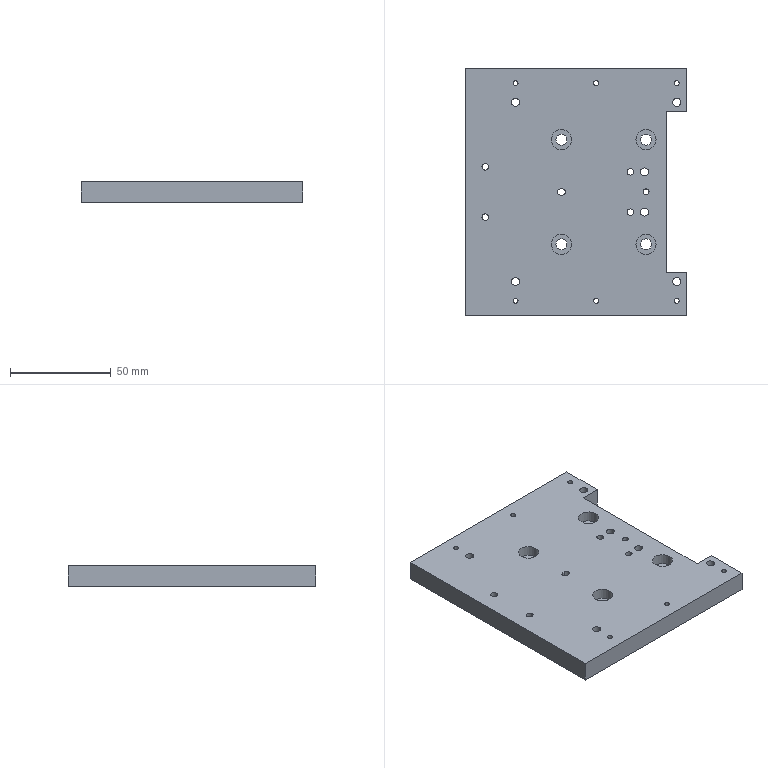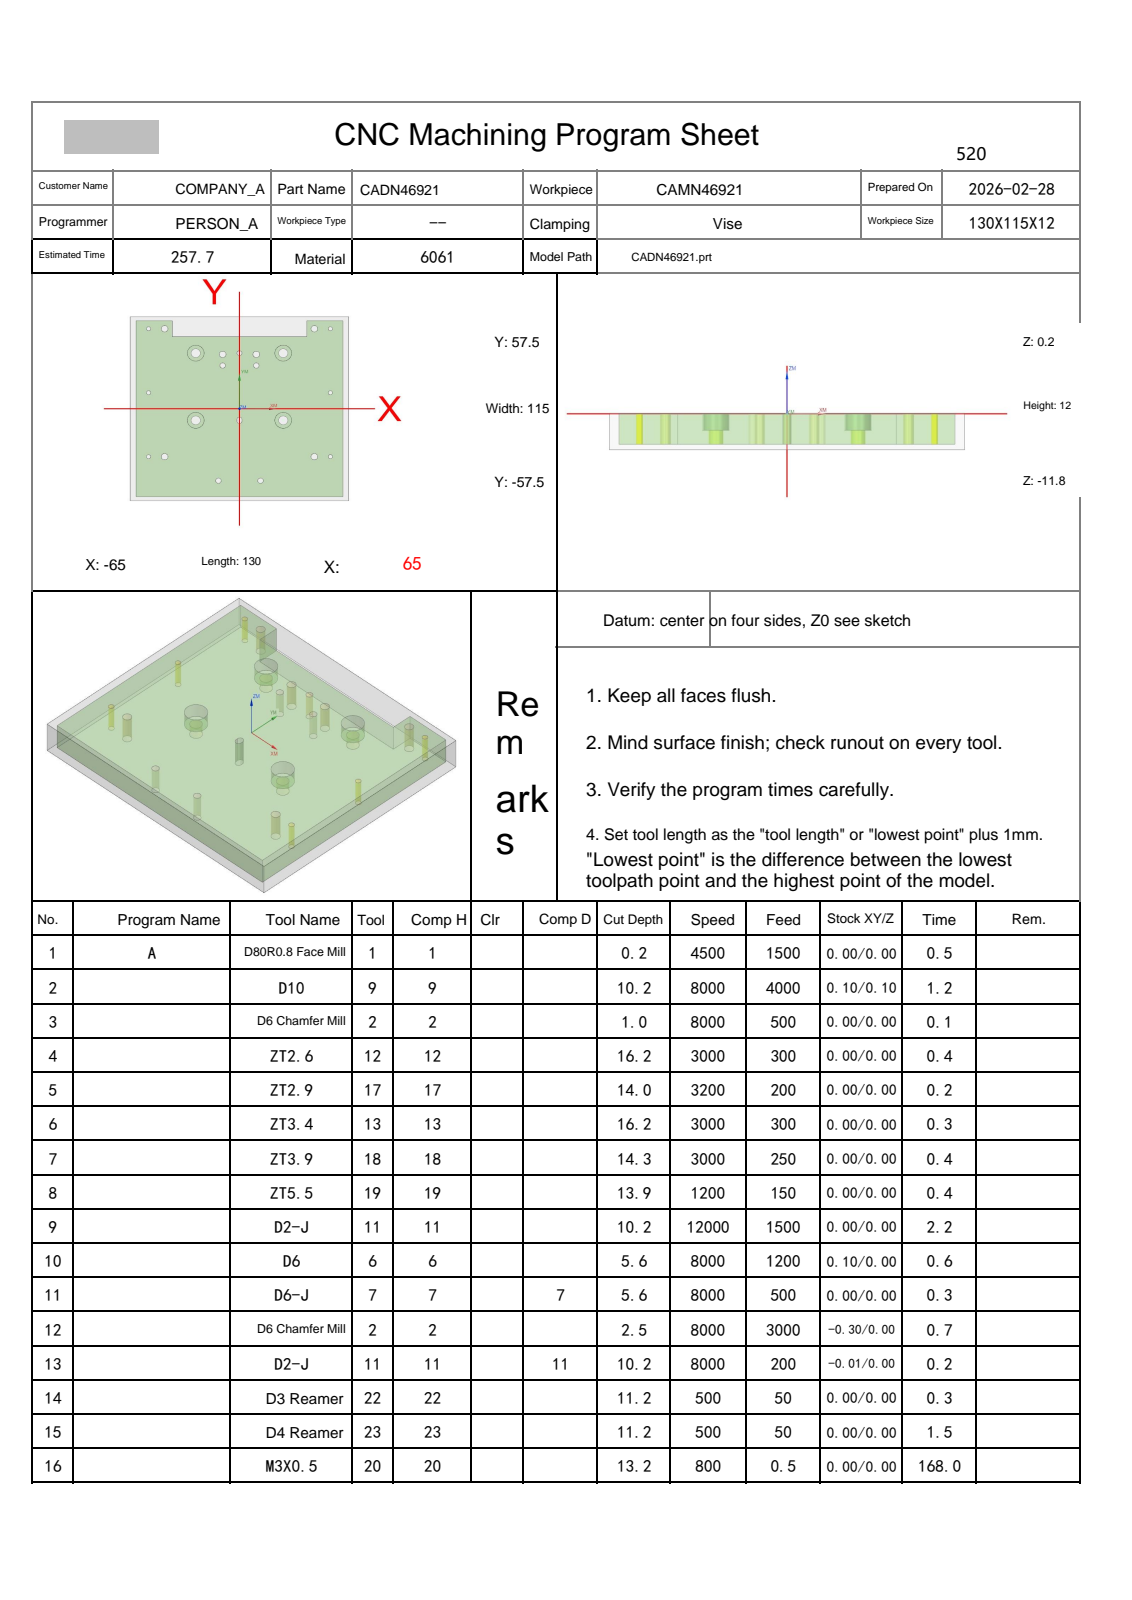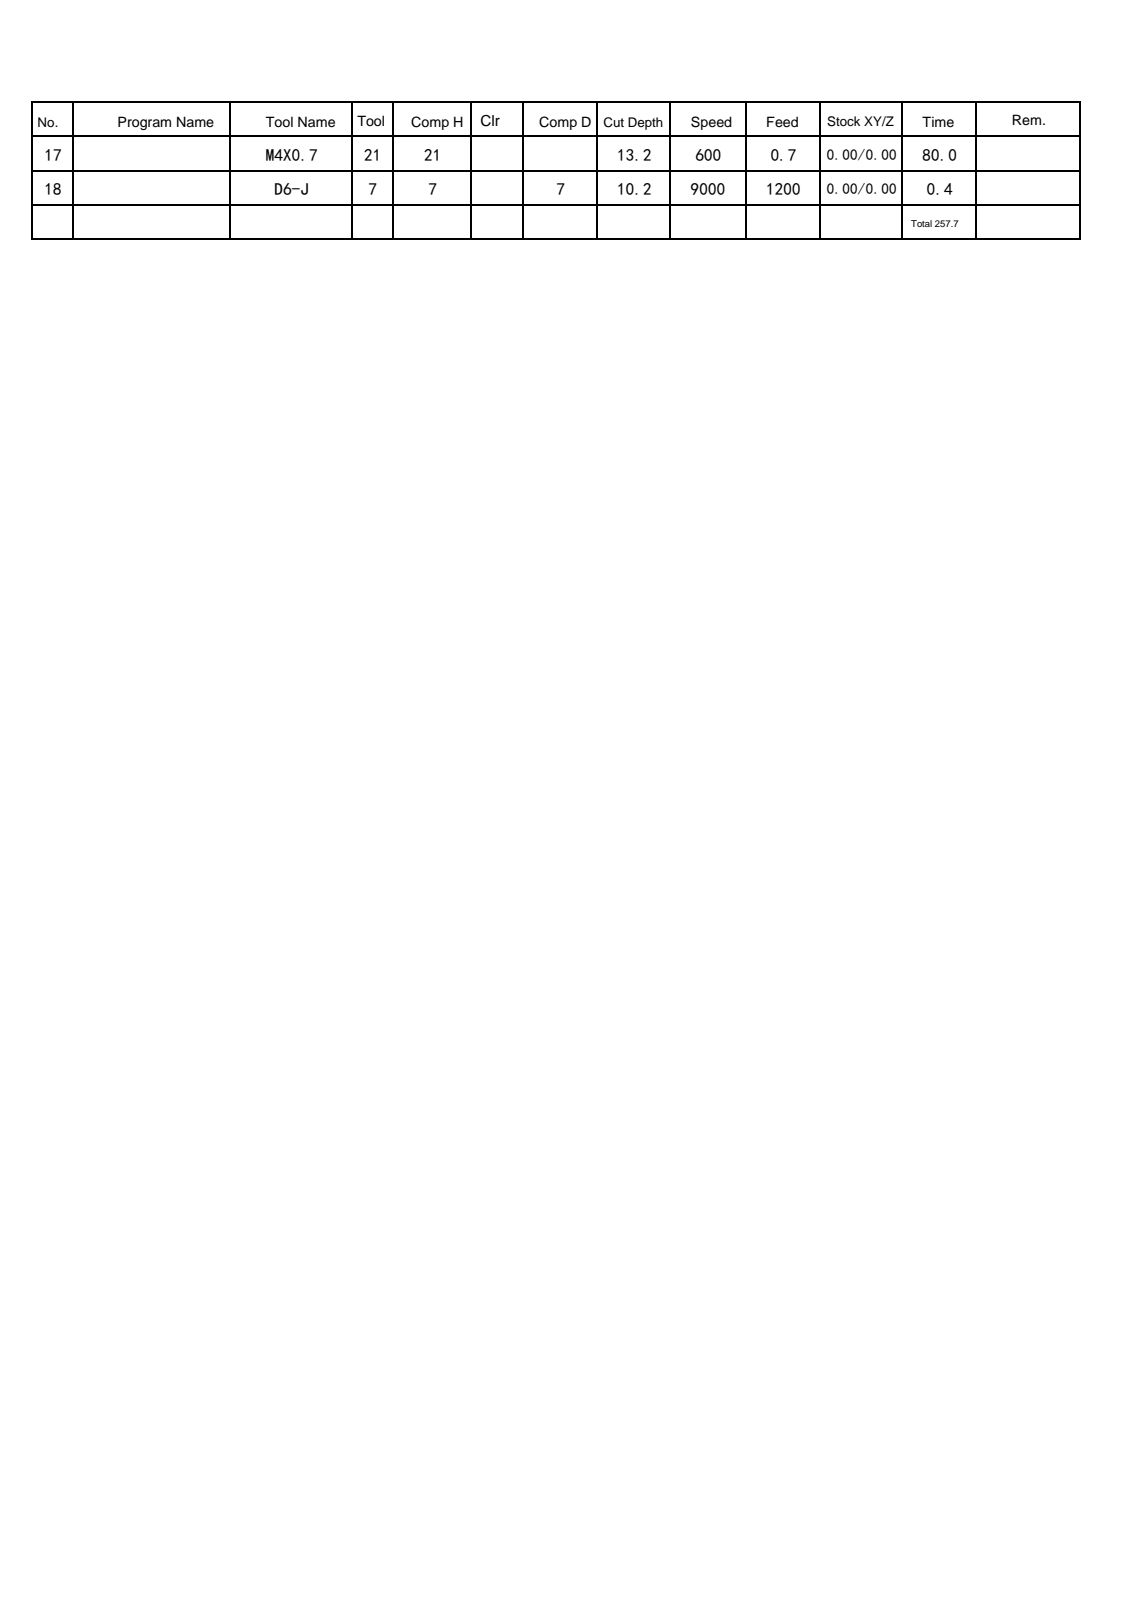NC program | NX | posted by the shop | part box 110 x 123 x 10 mm
Lines 1 to 794 of 4511:
%
O0001
(Machine time: 491.53 MIN)
(===Total Tool:15===)
(T1=D80R0.8 Face Mill D=80.  R=0.8  D-  H01 Z=-0.   )
(T9=D10     D=10.  R=0.   D-  H09 Z=-10.  )
(T2=D6 Chamfer Mill   D=6.   R=0.   D-  H02 Z=-2.3  )
(T12=ZT2.6  D=2.6  DR_a=118 D-  H12 Z=-16.  )
(T17=ZT2.9  D=2.9  DR_a=120 D-  H17 Z=-13.84)
(T13=ZT3.4  D=3.4  DR_a=118 D-  H13 Z=-16.  )
(T18=ZT3.9  D=3.9  DR_a=120 D-  H18 Z=-14.13)
(T19=ZT5.5  D=5.5  DR_a=118 D-  H19 Z=-13.65)
(T11=D2-J   D=2.   R=0.   D-  H11 Z=-10.  )
(T6=D6      D=6.   R=0.   D-  H06 Z=-5.4  )
(T7=D6-J    D=6.   R=0.   D7  H07 Z=-10.  )
(T22=D3 Reamer   D=3.   DR_a=180 D22 H22 Z=-11.  )
(T23=D4 Reamer   D=4.   DR_a=180 D-  H23 Z=-11.  )
(T20=M3X0.5 D=2.5  DR_a=180 D-  H20 Z=-13.  )
(T21=M4X0.7 D=3.3  DR_a=180 D-  H21 Z=-13.  )
G80 G90 G17 G49 G40
G91 G28 Z0
M01
N1 T01 M06
(D80R0.8 Face Mill  D=80. R=0.8 H=01 ce=0.00 di=0.00)
G00 G90 G54 X106.5 Y-47.5 M03 S4500
G43 H01 Z50.
M08
Z2.
G01 Z0.0 F1500.
X101.5
X-101.5
Y0.0
X101.5
Y47.5
X-101.5
X-106.5
Z2.
G00 Z50.
G91 G28 Z0.0
M05
M09
G91 G28 Z0.0
M01
N2 T09 M06
(D10  D=10. R=0. H=09 ce=0.10 di=0.10)
G00 G90 G54 X62.505 Y-68.93 M03 S8000
G43 H09 Z50.
M08
Z-8.
G01 X62.486 Y-68.832 Z-8.625 F4000.
X62.467 Y-68.734 Z-8.872
X62.448 Y-68.636 Z-9.054
X62.43 Y-68.538 Z-9.2
X62.411 Y-68.439 Z-9.323
X62.392 Y-68.341 Z-9.428
X62.374 Y-68.243 Z-9.52
X62.355 Y-68.145 Z-9.6
X62.336 Y-68.046 Z-9.67
X62.318 Y-67.948 Z-9.732
X62.299 Y-67.85 Z-9.786
X62.28 Y-67.752 Z-9.833
X62.261 Y-67.653 Z-9.874
X62.243 Y-67.555 Z-9.908
X62.224 Y-67.457 Z-9.936
X62.205 Y-67.359 Z-9.96
X62.187 Y-67.26 Z-9.977
X62.168 Y-67.162 Z-9.99
X62.149 Y-67.064 Z-9.997
X62.131 Y-66.966 Z-10.
X61.728 Y-64.851
G03 X61.47 Y-64.5 I-.505 J-.101
X57.665 Y-63.862 I-4.014 J-12.282
X48.447 Y-63.687 I-9.217 J-242.545
X45.931 Y-63.7 I0.0 J-242.72
G01 X-63.188 Y-63.681
G02 X-69.789 Y-59.121 I.026 J7.095
X-71.019 Y-52.954 I17.461 J6.69
X-71.212 Y-43.817 I217.094 J9.136
X-71.199 Y-41.437 I217.286 J0.0
G01 X-71.177 Y55.743
G02 X-66.615 Y62.297 I7.094 J-.073
X-60.526 Y63.515 I6.642 J-17.363
X-51.392 Y63.712 I9.134 J-212.235
X-49.009 Y63.699 I0.0 J-212.431
G01 X63.29 Y63.675
G02 X69.773 Y59.159 I-.116 J-7.078
X70.995 Y53.307 I-16.699 J-6.54
X71.216 Y43.947 I-197.872 J-9.36
X71.199 Y41.31 I-198.093 J0.0
G01 X71.175 Y-55.789
G02 X66.602 Y-62.298 I-7.094 J.123
X62.072 Y-63.143 I-4.53 J11.728
X61.502 Y-63.13 I0.0 J12.572
G03 X44.885 Y-62.897 I-16.617 J-593.259
X42.812 Y-62.901 I0.0 J-593.491
G01 X-61.328 Y-62.88
G02 X-68.312 Y-58.453 I.17 J7.991
X-70.034 Y-52.247 I15.045 J7.518
X-70.398 Y-43.651 I101.199 J8.596
X-70.39 Y-42.338 I101.564 J0.0
G01 X-70.376 Y53.887
G02 X-65.947 Y60.818 I7.979 J-.217
X-59.657 Y62.545 I7.553 J-15.196
X-51.066 Y62.899 I8.592 J-104.056
X-49.748 Y62.89 I0.0 J-104.41
G01 X61.347 Y62.878
G02 X68.339 Y58.403 I-.195 J-8.003
X70.05 Y52.108 I-15.333 J-7.548
X70.399 Y43.512 I-105.559 J-8.596
X70.391 Y42.198 I-105.908 J0.0
G01 X70.378 Y-53.847
G02 X65.26 Y-61.016 I-7.763 J.131
X59.223 Y-62.088 I-6.136 J17.023
X52.104 Y-62.14 I-7.119 J496.003
X46.088 Y-62.103 I0.0 J496.054
G01 X-59.568 Y-62.078
G02 X-67.383 Y-57.053 I.237 J8.959
X-69.224 Y-50.22 I16.92 J8.222
X-69.6 Y-40.954 I113.845 J9.266
X-69.591 Y-39.51 I114.221 J0.0
G01 X-69.579 Y51.99
G02 X-64.471 Y59.933 I8.996 J-.171
X-57.46 Y61.754 I8.273 J-17.449
X-47.647 Y62.11 I9.813 J-135.265
X-45.629 Y62.095 I0.0 J-135.62
G01 X59.55 Y62.077
G02 X67.333 Y57.147 I-.205 J-8.932
X69.203 Y50.405 I-16.458 J-8.195
X69.601 Y41.071 I-109.254 J-9.334
X69.59 Y39.537 I-109.652 J0.0
G01 X69.581 Y-51.963
G02 X64.414 Y-59.706 I-8.458 J.049
X58.127 Y-61.133 I-7.21 J17.206
X50.107 Y-61.327 I-8.02 J165.472
X47.368 Y-61.304 I0.0 J165.666
G01 X-57.808 Y-61.277
G02 X-62.753 Y-59.935 I.161 J10.372
G01 X-64.05 Y-59.417
X-65.106 Y-58.606
G02 X-67.093 Y-55.012 I8.097 J6.822
X-68.555 Y-47.093 I26.837 J9.048
X-68.814 Y-36.113 I232.394 J10.979
X-68.797 Y-33.337 I232.653 J0.0
G01 X-68.775 Y50.322
G02 X-66.234 Y56.812 I9.75 J-.075
G01 X-65.834 Y57.688
G02 X-63.98 Y59.456 I4.92 J-3.302
X-60.748 Y60.372 I4.831 J-10.887
X-50.156 Y61.25 I10.591 J-63.457
G01 X-49.837 Y61.249
X-37.837 Y61.298
X57.823 Y61.275
G02 X62.751 Y59.935 I-.18 J-10.397
G01 X64.05 Y59.417
X65.106 Y58.606
G02 X67.148 Y54.861 I-8.31 J-6.961
X68.566 Y46.933 I-27.584 J-9.022
X68.813 Y36.045 I-239.895 J-10.888
X68.797 Y33.337 I-240.142 J0.0
G01 X68.775 Y-50.322
G02 X66.395 Y-56.45 I-9.386 J.12
X65.02 Y-58.691 I-5.677 J1.941
X62.781 Y-59.936 I-3.933 J4.432
X53.648 Y-60.466 I-9.133 J78.497
G01 X53.498
X45.258 Y-60.501
X-55.922 Y-60.484
G02 X-59.036 Y-60.1 I.36 J15.741
G01 X-61.502
X-62.771 Y-59.933
X-61.502 Y-60.1
X61.5
G03 X63.98 Y-59.456 I-.213 J5.922
X65.834 Y-57.688 I-3.066 J5.071
X67.744 Y-51.783 I-20.321 J9.836
X68.146 Y-44.982 I-57.397 J6.801
X68.14 Y-44.199 I-57.799 J0.0
G01 X68.134 Y39.461
G03 X68.139 Y40.356 I-79.496 J.895
X67.562 Y49.917 I-79.501 J0.0
X66.6 Y54.052 I-26.021 J-3.876
X66.607 Y54.435 I-9.886 J.383
X66.426 Y56.32 I-9.894 J0.0
G01 X65.917 Y57.55
X66.426 Y56.32
G02 X66.624 Y53.695 I-17.291 J-2.625
X66.6 Y52.772 I-17.49 J0.0
X67.229 Y43.406 I-241.196 J-20.908
X67.366 Y30.259 I-629.886 J-13.147
X67.358 Y26.927 I-630.024 J0.0
G01 X67.334 Y-43.933
G02 X67.34 Y-44.665 I-46.782 J-.732
X66.871 Y-51.27 I-46.788 J0.0
G01 X66.6 Y-52.569
G02 X66.62 Y-53.631 I-28.416 J-1.062
X66.537 Y-55.798 I-28.436 J0.0
G01 X66.373 Y-56.499
G03 X66.6 Y-55.001 I-5.982 J1.672
G01 Y-54.736
G02 X66.708 Y-40.418 I945.397 J0.0
G01 X66.693 Y37.241
G02 X66.585 Y48.543 I590.334 J11.301
X66.6 Y52.803 I590.442 J0.0
G01 Y-48.957
G03 X67.1 Y-49.457 I.5 J0.0
X67.513 Y-49.239 I0.0 J.5
G01 X67.947 Y-48.602
X69.057 Y-46.972 Z-9.9
X69.65 Y-46.102
X69.687 Y-46.037
X69.715 Y-45.967
X69.731 Y-45.895
X69.737 Y-45.82
Y55.954
X69.73 Y56.211
X69.71 Y56.468
X69.677 Y56.724
X69.631 Y56.977
X69.571 Y57.228
X69.499 Y57.475
X69.414 Y57.718
X69.316 Y57.957
X69.206 Y58.19
X69.085 Y58.417
X68.951 Y58.638
X68.807 Y58.851
X68.652 Y59.057
X67.036 Y61.084
X66.983 Y61.141
X66.921 Y61.189
X66.853 Y61.227
X66.78 Y61.253
X66.703 Y61.268
X66.625 Y61.271
X66.548 Y61.262
X66.473 Y61.241
X65.994 Y61.066
X64.144 Y60.386 Z-10.
X62.911 Y59.94
X59.239 Y60.42
G03 X50.912 Y60.673 I-8.327 J-136.576
X48.684 Y60.655 I0.0 J-136.83
G01 X-45.841 Y60.645
G03 X-47.114 Y60.652 I-1.274 J-108.167
X-57.504 Y60.152 I0.0 J-108.175
G01 X-57.928 Y60.1
X-61.498
X-62.781 Y59.936
X-61.498 Y60.1
X-39.725 Y60.075
G03 X-31.255 Y59.847 I8.47 J156.731
X-29.209 Y59.86 I0.0 J156.96
G01 X38.547 Y59.878
G02 X40.002 Y60.1 I3.204 J-16.087
G01 X61.502
X62.295 Y59.995
X62.36 Y59.991
G03 X62.86 Y60.491 I0.0 J.5
X62.623 Y60.916 I-.5 J0.0
G01 X61.653 Y61.517
X59.977 Y62.556 Z-9.9
X59.8 Y62.665
X59.742 Y62.696
X59.68 Y62.719
X59.616 Y62.734
X59.55 Y62.74
X40.521 Y63.247
X40.436 Y63.242
X40.353 Y63.222
X40.275 Y63.189
X40.203 Y63.143
X40.14 Y63.086
X40.088 Y63.019
X40.048 Y62.944
X39.893 Y62.583
X39.115 Y60.771 Z-10.
X38.812 Y60.081
G02 X37.832 Y59.658 I-1.101 J1.202
X32.456 Y59.247 I-5.376 J34.946
X31.849 Y59.252 I0.0 J35.358
G01 X22.871 Y59.218
X-33.56 Y59.243
X-37.29 Y59.346
X-38.68 Y59.926
X-39.998 Y60.1
X-38.68 Y59.926
G03 X-36.585 Y59.055 I11.251 J24.099
X-31.218 Y58.497 I5.367 J25.538
G01 X-31.088
G03 X-20.883 Y58.417 I10.205 J646.307
X-19.532 Y58.418 I0.0 J646.388
G01 X30.574 Y58.444
G03 X31.065 Y58.441 I.492 J44.925
X36.555 Y58.778 I0.0 J44.928
X37.45 Y59.417 I-3.02 J5.179
G01 X38.485 Y59.845
G03 X36.58 Y58.757 I1.486 J-4.809
G02 X33.107 Y58.014 I-3.831 J9.425
X24.641 Y57.766 I-8.466 J144.323
X22.707 Y57.779 I0.0 J144.571
G01 X-27.719 Y57.804
G02 X-28.459 Y57.798 I-.74 J51.357
X-35.172 Y58.239 I0.0 J51.362
X-36.394 Y58.606 I.167 J2.77
G01 X-37.409 Y59.385
G03 X-35.849 Y58.211 I9.538 J11.048
X-31.824 Y57.286 I4.687 J11.178
X-23.321 Y56.978 I8.503 J117.162
X-22.001 Y56.985 I0.0 J117.47
G01 X26.58 Y57.001
G03 X27.394 Y56.995 I.814 J51.142
X34.203 Y57.45 I0.0 J51.148
X35.877 Y57.95 I-.524 J4.802
G02 X36.648 Y58.801 I3.084 J-2.019
G03 X35.817 Y57.87 I2.562 J-3.122
G02 X32.885 Y56.843 I-3.666 J5.766
X25.432 Y56.36 I-7.453 J57.247
X24.665 Y56.365 I0.0 J57.73
G01 X-22.542 Y56.35
G02 X-23.837 Y56.34 I-1.295 J84.158
X-32.198 Y56.757 I0.0 J84.168
X-35.682 Y57.718 I.883 J9.996
G01 X-36.355 Y58.556
G03 X-35.092 Y57.208 I3.927 J2.413
X-31.072 Y56.023 I5.06 J9.756
X-22.39 Y55.553 I8.681 J79.953
X-21.422 Y55.559 I0.0 J80.422
G01 X23.938 Y55.564
G03 X24.727 Y55.558 I.789 J57.881
X32.378 Y56.066 I0.0 J57.886
X35.293 Y57.018 I-1.102 J8.313
X35.583 Y57.55 I-1.475 J1.151
G01 X35.875 Y57.931
G03 X35.374 Y57.065 I1.947 J-1.707
G02 X32.939 Y55.801 I-3.455 J3.676
X26.378 Y55.018 I-6.847 J29.497
X16.15 Y54.895 I-10.228 J425.475
X14.228 Y54.899 I0.0 J425.598
G01 X-21.483 Y54.924
G02 X-22.293 Y54.919 I-.809 J72.281
X-30.925 Y55.436 I0.0 J72.285
X-34.897 Y56.658 I1.245 J11.119
X-35.583 Y57.55 I.614 J1.182
G01 X-35.681 Y57.677
G02 X-35.32 Y56.926 I-3.681 J-2.23
G03 X-33.019 Y55.424 I3.621 J3.034
X-26.761 Y54.346 I7.101 J22.511
X-16.524 Y54.093 I10.237 J206.976
X-14.649 Y54.101 I0.0 J207.229
G01 X21.698 Y54.126
G03 X22.408 Y54.122 I.711 J65.855
X30.737 Y54.651 I0.0 J65.858
X34.774 Y56.016 I-1.098 J9.897
X35.074 Y56.32 I-2.438 J2.705
G01 X35.441 Y57.207
G02 X34.923 Y56.066 I-4.848 J1.512
X32.248 Y54.565 I-4.032 J4.054
X25.829 Y53.643 I-7.141 J26.887
X15.924 Y53.454 I-9.905 J260.528
X14.148 Y53.46 I0.0 J260.716
G01 X-19.322 Y53.486
G02 X-20.139 Y53.481 I-.816 J78.127
X-29.49 Y54.043 I0.0 J78.132
X-34.258 Y55.54 I1.366 J12.694
X-35.074 Y56.32 I.733 J1.583
G01 X-35.38 Y57.059
G03 X-34.85 Y55.836 I6.316 J2.011
X-31.93 Y54.043 I4.58 J4.184
X-24.941 Y52.904 I7.952 J26.768
X-12.517 Y52.637 I12.424 J289.718
X-8.892 Y52.66 I0.0 J289.984
G01 X19.934 Y52.69
G03 X20.601 Y52.687 I.667 J68.704
X29.603 Y53.279 I0.0 J68.708
X34.042 Y54.754 I-1.455 J11.799
X34.994 Y55.713 I-.967 J1.912
G01 X35.074 Y56.32
Y56.271
G02 X34.182 Y54.6 I-2.011 J0.0
X29.919 Y52.853 I-5.859 J8.225
X21.099 Y52.093 I-8.82 J50.778
G01 X21.09
X12.549 Y52.02
X-17.402 Y52.048
G02 X-18.149 Y52.044 I-.747 J85.721
X-28.074 Y52.621 I0.0 J85.724
X-33.372 Y54.176 I1.684 J15.538
X-34.972 Y55.605 I1.598 J3.398
G01 X-35.074 Y56.32
Y56.314
G03 X-33.953 Y54.175 I2.602 J0.0
X-29.412 Y52.234 I6.527 J8.987
X-20.52 Y51.337 I9.338 J48.079
X-9.772 Y51.22 I11.644 J577.468
G01 X18.173 Y51.252
G03 X18.776 Y51.25 I.602 J75.544
X28.35 Y51.859 I0.0 J75.546
X33.518 Y53.519 I-1.643 J13.992
X34.868 Y54.781 I-1.808 J3.286
G01 X34.984 Y55.636
G02 X34.814 Y54.568 I-3.95 J.082
X32.508 Y52.601 I-4.19 J2.574
X26.353 Y51.058 I-7.671 J17.558
X15.687 Y50.584 I-10.666 J119.748
X14.208 Y50.593 I0.0 J120.222
G01 X-15.18 Y50.607
G02 X-16.067 Y50.602 I-.887 J96.053
X-26.963 Y51.222 I0.0 J96.058
X-32.769 Y52.896 I1.904 J17.516
X-34.874 Y54.772 I2.044 J4.412
G01 X-34.983 Y55.633
G03 X-34.774 Y54.376 I4.726 J.142
X-32.255 Y52.125 I4.726 J2.753
X-25.853 Y50.395 I8.298 J18.003
G01 X-22.925 Y50.1
X23.646 Y50.123
G03 X31.233 Y51.408 I-.56 J26.332
X34.563 Y53.509 I-2.269 J7.284
X34.9 Y54.135 I-1.094 J.994
G01 Y54.855
G02 X34.925 Y54.506 I-2.424 J-.349
X34.745 Y53.583 I-2.449 J0.0
X32.224 Y51.407 I-4.761 J2.965
X28.178 Y50.1 I-6.943 J14.582
G01 X23.058
X29.646 Y50.125
G03 X34.562 Y52.602 I-.644 J7.395
X34.9 Y53.234 I-1.322 J1.114
G01 Y54.114
G02 X34.921 Y53.713 I-3.914 J-.401
X34.829 Y52.867 I-3.935 J0.0
X32.55 Y50.629 I-4.308 J2.106
X31.261 Y50.1 I-4.205 J8.411
G01 X29.261
G03 X30.191 Y50.082 I.93 J23.649
X31.947 Y50.147 I0.0 J23.667
X34.866 Y52.224 I-.866 J4.307
X34.901 Y53.062 I-10.028 J.838
G01 X34.9 Y53.185
G02 X34.923 Y52.793 I-3.34 J-.392
X34.836 Y52.034 I-3.363 J0.0
X32.676 Y50.1 I-3.265 J1.474
G01 X31.556
G03 X32.08 Y50.08 I.524 J6.804
X33.219 Y50.176 I0.0 J6.824
X34.878 Y51.543 I-.826 J2.692
G01 X34.9 Y52.372
G02 X34.921 Y52.034 I-2.688 J-.339
X34.816 Y51.287 I-2.709 J0.0
X33.487 Y50.1 I-2.002 J.903
G01 X32.767
G03 X33.112 Y50.081 I.345 J3.107
X33.985 Y50.205 I0.0 J3.127
X34.9 Y51.155 I-.451 J1.35
G01 Y51.635
G02 X34.924 Y51.382 I-1.308 J-.253
X33.954 Y50.1 I-1.332 J0.0
G01 X33.554
G03 X33.796 Y50.076 I.243 J1.223
X34.867 Y50.684 I0.0 J1.247
G01 X34.9 Y51.118
X34.923 Y50.925
G02 X34.088 Y50.09 I-.835 J0.0
G01 X33.96 Y50.1
X34.146 Y50.078
G03 X34.807 Y50.435 I0.0 J.79
X34.891 Y50.728 I-.467 J.293
X34.34 Y51.279 I-.551 J0.0
X33.789 Y50.728 I0.0 J-.551
G01 X33.792 Y50.672
G03 X34.342 Y50.121 I.55 J0.0
G01 X34.45 Y50.132
G03 X34.912 Y50.744 I-.175 J.613
G01 X34.9 Y50.867
G03 X34.625 Y51.313 I-.504 J-.003
G01 X33.907 Y51.675
X32.146 Y52.562 Z-9.9
X31.763 Y52.754
X31.691 Y52.784
X31.616 Y52.802
X31.538 Y52.808
X-20.18 Y52.845
X-20.253 Y52.84
X-20.325 Y52.824
X-20.393 Y52.797
X-20.457 Y52.762
X-20.515 Y52.717
X-20.566 Y52.664
X-20.64 Y52.574
X-21.898 Y51.056 Z-10.
X-22.591 Y50.228
G02 X-22.925 Y50.1 I-.344 J.398
X-24.286 Y50.077 I-1.361 J40.414
X-27.449 Y50.201 I0.0 J40.437
X-33.35 Y52.289 I1.283 J13.008
X-34.885 Y54.044 I2.382 J3.632
G01 X-34.9 Y54.854
G03 X-34.924 Y54.483 I2.8 J-.37
X-33.942 Y52.342 I2.824 J0.0
X-29.808 Y50.1 I6.491 J7.036
G01 X-26.048
G02 X-27.717 Y50.078 I-1.669 J62.67
X-30.515 Y50.14 I0.0 J62.692
X-34.805 Y52.97 I.933 J6.083
X-34.924 Y53.71 I2.262 J.74
X-34.9 Y54.044 I2.38 J0.0
G03 X-34.925 Y53.65 I3.115 J-.394
X-34.66 Y52.388 I3.14 J0.0
X-31.867 Y50.1 I4.503 J2.648
G01 X-30.107
G02 X-30.725 Y50.093 I-.618 J27.81
X-32.204 Y50.132 I0.0 J27.817
X-34.884 Y52.313 I.915 J3.861
G01 X-34.9 Y53.205
G03 X-34.924 Y52.804 I3.304 J-.4
X-34.746 Y51.729 I3.328 J0.0
X-32.982 Y50.1 I2.736 J1.193
G01 X-31.942
G02 X-32.402 Y50.082 I-.46 J5.895
X-33.338 Y50.157 I0.0 J5.913
X-34.9 Y51.675 I.727 J2.311
G01 Y52.315
G03 X-34.924 Y51.988 I2.202 J-.327
X-34.594 Y50.822 I2.226 J0.0
X-33.672 Y50.1 I1.396 J.834
G01 X-33.032
G02 X-33.337 Y50.08 I-.305 J2.345
X-34.032 Y50.185 I0.0 J2.365
X-34.913 Y51.458 I.48 J1.273
G01 X-34.9 Y51.647
G03 X-34.924 Y51.381 I1.433 J-.266
X-34.235 Y50.142 I1.457 J0.0
X-33.725 Y50.1 I.51 J3.011
G01 X-33.681
G02 X-33.894 Y50.078 I-.213 J1.038
X-34.9 Y50.807 I0.0 J1.059
G01 Y51.127
G03 X-34.922 Y50.928 I.886 J-.199
X-34.517 Y50.172 I.908 J0.0
X-34.257 Y50.107 I.26 J.485
X-33.707 Y50.657 I0.0 J.55
X-33.907 Y51.081 I-.55 J0.0
X-34.333 Y51.273 I-.426 J-.374
X-34.868 Y50.894 I0.0 J-.567
G01 X-34.887 Y50.737
G03 X-34.226 Y50.077 I.66 J0.0
G01 X-34.053 Y50.1
G03 X-33.609 Y50.371 I-.003 J.504
G01 X-33.34 Y50.894
X-32.438 Y52.647 Z-9.9
X-31.89 Y53.713
X-31.86 Y53.786
X-31.841 Y53.863
X-31.835 Y53.942
Y57.384
X-31.842 Y57.601
X-31.861 Y57.817
X-31.894 Y58.031
X-31.939 Y58.243
X-31.998 Y58.452
X-32.068 Y58.657
X-32.151 Y58.858
X-32.246 Y59.053
X-32.353 Y59.241
X-32.47 Y59.424
X-32.599 Y59.598
X-32.738 Y59.765
X-32.886 Y59.923
X-35.713 Y62.749
X-35.871 Y62.898
X-36.037 Y63.037
X-36.212 Y63.165
X-36.394 Y63.283
X-36.583 Y63.389
X-36.778 Y63.484
X-36.978 Y63.567
X-37.183 Y63.638
X-37.392 Y63.696
X-37.604 Y63.742
X-37.819 Y63.774
X-38.034 Y63.794
X-38.251 Y63.801
X-62.09
X-62.355 Y63.794
X-62.619 Y63.774
X-62.881 Y63.741
X-63.142 Y63.694
X-63.4 Y63.634
X-63.654 Y63.562
X-63.905 Y63.476
X-64.151 Y63.378
X-64.391 Y63.268
X-64.626 Y63.146
X-64.854 Y63.012
X-65.076 Y62.867
X-65.289 Y62.711
X-67.382 Y61.098
X-67.442 Y61.043
X-67.492 Y60.98
X-67.531 Y60.91
X-67.559 Y60.834
X-67.574 Y60.755
X-67.576 Y60.674
X-67.565 Y60.594
X-67.541 Y60.517
X-67.279 Y59.856
X-66.55 Y58.024 Z-10.
X-66.2 Y57.128
Y57.123
G02 X-66.396 Y56.439 I-1.29 J0.0
G03 X-68.045 Y48.503 I19.269 J-8.142
X-68.168 Y38.925 I371.269 J-9.577
X-68.158 Y36.184 I371.392 J0.0
G01 X-68.134 Y-39.476
G03 X-68.139 Y-40.339 I80.079 J-.863
X-67.572 Y-49.853 I80.084 J0.0
X-66.6 Y-54.048 I25.668 J3.737
X-66.608 Y-54.433 I9.899 J-.386
X-66.426 Y-56.32 I9.906 J0.0
G01 X-65.917 Y-57.55
X-66.426 Y-56.32
G02 X-66.624 Y-53.692 I17.323 J2.628
X-66.6 Y-52.768 I17.521 J0.0
X-67.248 Y-42.82 I221.247 J19.403
X-67.363 Y-29.751 I738.773 J13.069
X-67.358 Y-26.821 I738.888 J0.0
G01 X-67.334 Y43.959
G02 X-67.34 Y44.688 I47.486 J.729
X-66.878 Y51.297 I47.492 J0.0
G01 X-66.6 Y52.645
G02 X-66.619 Y53.666 I27.808 J1.022
X-66.537 Y55.8 I27.826 J0.0
G01 X-66.369 Y56.515
G03 X-66.6 Y55.001 I6.017 J-1.69
G01 Y54.692
G02 X-66.708 Y40.62 I-917.145 J0.0
G01 X-66.692 Y-37.28
G02 X-66.584 Y-48.527 I-585.098 J-11.247
X-66.6 Y-52.801 I-585.206 J0.0
G01 Y48.959
G03 X-67.047 Y49.461 I-.506 J-.001
G01 X-69.065 Y49.695
X-69.164 Y49.706 Z-9.997
X-69.263 Y49.718 Z-9.99
X-69.363 Y49.729 Z-9.977
X-69.462 Y49.741 Z-9.96
X-69.561 Y49.752 Z-9.936
X-69.661 Y49.764 Z-9.908
X-69.76 Y49.775 Z-9.874
X-69.859 Y49.787 Z-9.833
X-69.959 Y49.798 Z-9.786
X-70.058 Y49.81 Z-9.732
X-70.157 Y49.821 Z-9.67
X-70.257 Y49.833 Z-9.6
X-70.356 Y49.844 Z-9.52
X-70.455 Y49.856 Z-9.428
X-70.555 Y49.867 Z-9.323
X-70.654 Y49.879 Z-9.2
X-70.753 Y49.89 Z-9.054
X-70.853 Y49.902 Z-8.872
X-70.952 Y49.913 Z-8.625
X-71.051 Y49.925 Z-8.
G00 Z50.
G91 G28 Z0.0
M05
M09
G91 G28 Z0.0
M01
N3 T02 M06
(D6 Chamfer Mill  D=6. R=0. H=02 ce=0.00 di=0.10)
G00 G90 G54 X-12.5 Y-45. M03 S8000
G43 H02 Z50.
M08
G98 G81 X-12.5 Y-45. Z-.8 R1. F500.
X12.5
X44.5 Y-30.
X54.
X26. Y-7.25
X54. Y10.
Y50.
X44.5
X26. Y34.75
X10. Y27.
Y34.
X0.0 Y34.75
X-10. Y34.
Y27.
X-26. Y34.75
X-44.5 Y50.
X-54.
Y10.
X-26. Y-7.25
X-44.5 Y-30.
X-54.
G80
G00 Z50.
G00 G90 X0.0 Y-6.75 M03 S8000
Z50.
G98 G81 X0.0 Y-6.75 Z-.8 R1. F500.
G80
G00 Z50.
G91 G28 Z0.0
M05
M09
G91 G28 Z0.0
M01
N4 T12 M06
(ZT2.6 D=2.6 DR_a=118 H=12)
G00 G90 G54 X54. Y50. M03 S3000
G43 H12 Z50.
M08
G98 G83 X54. Y50. Z-16. R1. F300. Q2.
Y10.
Y-30.
X-54.
Y10.
Y50.
G80
G00 Z50.
G91 G28 Z0.0
M05
M09
G91 G28 Z0.0
M01
N5 T17 M06
(ZT2.9 D=2.9 DR_a=120 H=17)
G00 G90 G54 X0.0 Y34.75 M03 S3200
G43 H17 Z50.
M08
G98 G83 X0.0 Y34.75 Z-13.837 R1. F200. Q2.
G80
G00 Z50.
G00 G90 X0.0 Y-6.75 M03 S3200
Z50.
G98 G83 X0.0 Y-6.75 Z-13.837 R1. F200. Q2.
G80
G00 Z50.
G91 G28 Z0.0
M05
M09
G91 G28 Z0.0
M01
N6 T13 M06
(ZT3.4 D=3.4 DR_a=118 H=13)
G00 G90 G54 X12.5 Y-45. M03 S3000
G43 H13 Z50.
M08
G98 G83 X12.5 Y-45. Z-16. R1. F300. Q2.
X-12.5
X-10. Y27.
X10.
G80
G00 Z50.
G91 G28 Z0.0
M05
M09
G91 G28 Z0.0
M01
N7 T18 M06
(ZT3.9 D=3.9 DR_a=120 H=18)
G00 G90 G54 X44.5 Y-30. M03 S3000
G43 H18 Z50.
M08
G98 G83 X44.5 Y-30. Z-14.126 R1. F250. Q2.
Y50.
X10. Y34.
X-10.
X-44.5 Y50.
Y-30.
G80
G00 Z50.
G91 G28 Z0.0
M05
M09
G91 G28 Z0.0
M01
N8 T19 M06
(ZT5.5 D=5.5 DR_a=118 H=19)
G00 G90 G54 X26. Y34.75 M03 S1200
G43 H19 Z50.
M08
G98 G83 X26. Y34.75 Z-13.652 R1. F150. Q2.
Y-7.25
X-26.
Y34.75
G80
G00 Z50.
G91 G28 Z0.0
M05
M09
G91 G28 Z0.0
M01